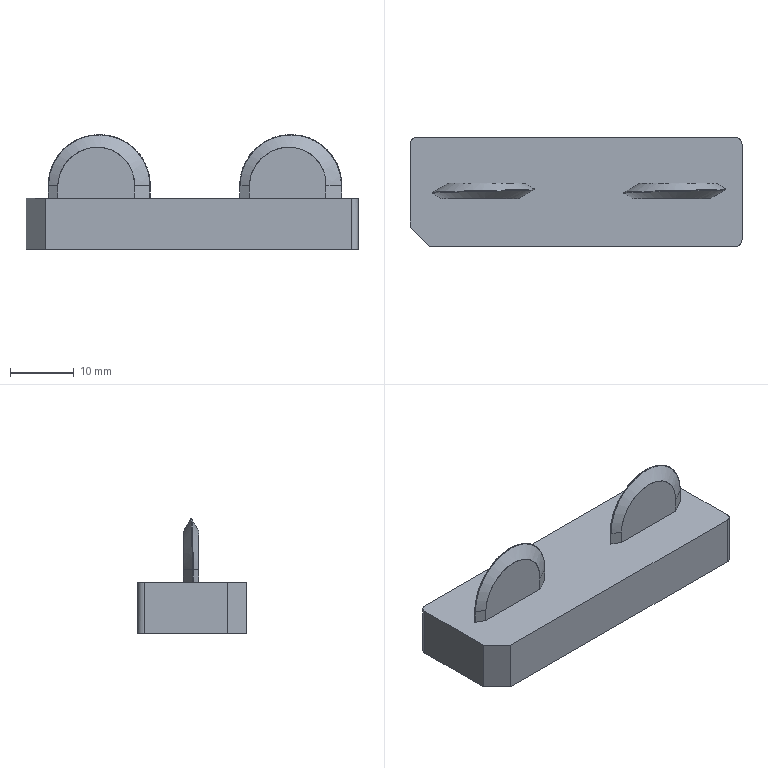NC program | PowerMill | posted with a generic post | part box 52 x 17 x 17.993 mm
Lines 4776 to 5766 of 175197:
N4873 M6
N4874 S18000 M03
N4875 G00 G90 X0.0 Y0.0
N4876 G43 Z9.812 H2
N4877
N4878 G05 P10000 R4
N4879 X-15.0046 Y3.2741
N4880 Z0.8142
N4881 G01 Z-0.3858 F3600.0
N4882 X-15.0151 Y3.2548 F6000.0
N4883 G03 X-14.9363 Y2.9861 I0.1738 J-0.0949
N4884 G01 X-13.6655 Y2.292
N4885 X-12.9334 Y2.2654
N4886 X-12.4453 Y2.2003
N4887 X-11.9573 Y2.0481
N4888 X-11.4692 Y1.7468
N4889 X-11.0258 Y1.2201
N4890 X-10.8183 Y0.7321
N4891 X-10.7493 Y0.244
N4892 X-10.7885 Y-0.244
N4893 X-10.9561 Y-0.7321
N4894 X-11.2918 Y-1.2201
N4895 X-11.4692 Y-1.3848
N4896 X-12.0007 Y-1.7082
N4897 X-12.4453 Y-1.8465
N4898 X-13.4214 Y-1.9746
N4899 X-14.3976 Y-2.0349
N4900 X-15.3737 Y-2.0324
N4901 X-16.3498 Y-1.9659
N4902 X-16.8378 Y-1.8637
N4903 X-17.3259 Y-1.6487
N4904 X-17.8296 Y-1.2201
N4905 X-18.1298 Y-0.7321
N4906 X-18.2691 Y-0.244
N4907 X-18.2928 Y0.244
N4908 X-18.2024 Y0.7321
N4909 X-17.974 Y1.2201
N4910 X-17.8139 Y1.4288
N4911 X-17.5262 Y1.7082
N4912 X-17.3259 Y1.8456
N4913 X-16.8378 Y2.0588
N4914 X-16.3498 Y2.1713
N4915 X-15.3737 Y2.2743
N4916 X-14.3976 Y2.3185
N4917 X-13.6655 Y2.292
N4918 X-15.0119 Y3.3954 Z-0.5837
N4919 X-15.0224 Y3.3761
N4920 G03 X-14.9438 Y3.1073 I0.1737 J-0.0951
N4921 G01 X-13.6613 Y2.4056
N4922 X-12.9334 Y2.3787
N4923 X-11.9573 Y2.2695
N4924 X-11.5961 Y2.1962
N4925 X-10.9812 Y1.929
N4926 X-10.6898 Y1.7082
N4927 X-10.4931 Y1.5014
N4928 X-10.2976 Y1.2201
N4929 X-10.1004 Y0.7321
N4930 X-10.0369 Y0.244
N4931 X-10.0778 Y-0.244
N4932 X-10.2499 Y-0.7321
N4933 X-10.5936 Y-1.2201
N4934 X-10.9812 Y-1.5344
N4935 X-11.3257 Y-1.7082
N4936 X-11.9573 Y-1.8834
N4937 X-13.4214 Y-2.087
N4938 X-14.3976 Y-2.149
N4939 X-15.3737 Y-2.1462
N4940 X-16.3498 Y-2.0801
N4941 X-17.3259 Y-1.9508
N4942 X-17.8139 Y-1.7872
N4943 X-17.9761 Y-1.7082
N4944 X-18.302 Y-1.4802
N4945 X-18.5591 Y-1.2201
N4946 X-18.79 Y-0.8714
N4947 X-18.8554 Y-0.7321
N4948 X-18.9931 Y-0.244
N4949 X-19.011 Y0.244
N4950 X-18.9164 Y0.7321
N4951 X-18.79 Y1.028
N4952 X-18.6799 Y1.2201
N4953 X-18.302 Y1.6425
N4954 X-17.8139 Y1.9476
N4955 X-17.3259 Y2.1163
N4956 X-16.3498 Y2.2825
N4957 X-15.3737 Y2.3875
N4958 X-14.3976 Y2.4329
N4959 X-13.6613 Y2.4056
N4960 X-14.9389 Y3.5136 Z-0.7815
N4961 X-14.9498 Y3.4945
N4962 G03 X-14.8755 Y3.2245 I0.1721 J-0.0978
N4963 G01 X-13.6546 Y2.5304
N4964 X-12.9334 Y2.492
N4965 X-11.9573 Y2.3804
N4966 X-10.9812 Y2.1908
N4967 X-10.4931 Y1.9775
N4968 X-10.1335 Y1.7082
N4969 X-10.0051 Y1.578
N4970 X-9.7514 Y1.2201
N4971 X-9.5544 Y0.7321
N4972 X-9.4932 Y0.244
N4973 X-9.5391 Y-0.244
N4974 X-9.7152 Y-0.7321
N4975 X-10.0051 Y-1.1528
N4976 X-10.4931 Y-1.5541
N4977 X-10.9812 Y-1.7729
N4978 X-11.9573 Y-1.992
N4979 X-13.3897 Y-2.1962
N4980 X-14.3976 Y-2.263
N4981 X-15.3737 Y-2.26
N4982 X-16.3095 Y-2.1962
N4983 X-17.8139 Y-1.9796
N4984 X-18.302 Y-1.8246
N4985 X-18.543 Y-1.7082
N4986 X-18.79 Y-1.5381
N4987 X-19.1129 Y-1.2201
N4988 X-19.2781 Y-0.9765
N4989 X-19.404 Y-0.7321
N4990 X-19.5376 Y-0.244
N4991 X-19.5511 Y0.244
N4992 X-19.4525 Y0.7321
N4993 X-19.213 Y1.2201
N4994 X-18.79 Y1.6717
N4995 X-18.302 Y1.9596
N4996 X-17.8139 Y2.1187
N4997 X-16.8378 Y2.3122
N4998 X-15.8617 Y2.4504
N4999 X-14.8856 Y2.5294
N5000 X-13.9095 Y2.544
N5001 X-13.6546 Y2.5304
N5002 X-15.0246 Y3.6221 Z-0.9794
N5003 X-15.0349 Y3.6026
N5004 G03 X-14.9531 Y3.3348 I0.1748 J-0.0929
N5005 G01 X-13.6518 Y2.6428
N5006 X-13.4214 Y2.637
N5007 X-12.4453 Y2.5528
N5008 X-11.4692 Y2.4064
N5009 X-10.4951 Y2.1962
N5010 X-10.0051 Y1.9658
N5011 X-9.6708 Y1.7082
N5012 X-9.517 Y1.5445
N5013 X-9.2943 Y1.2201
N5014 X-9.1039 Y0.7321
N5015 X-9.0457 Y0.244
N5016 X-9.094 Y-0.244
N5017 X-9.2715 Y-0.7321
N5018 X-9.517 Y-1.0997
N5019 X-9.6267 Y-1.2201
N5020 X-10.0051 Y-1.521
N5021 X-10.3719 Y-1.7082
N5022 X-10.9812 Y-1.8864
N5023 X-11.9573 Y-2.1006
N5024 X-12.5186 Y-2.1962
N5025 X-13.9095 Y-2.352
N5026 X-14.8856 Y-2.3811
N5027 X-15.8617 Y-2.345
N5028 X-16.8378 Y-2.2461
N5029 X-18.302 Y-1.9865
N5030 X-18.79 Y-1.8218
N5031 X-19.0097 Y-1.7082
N5032 X-19.2781 Y-1.5193
N5033 X-19.5727 Y-1.2201
N5034 X-19.7661 Y-0.9242
N5035 X-19.8572 Y-0.7321
N5036 X-19.9873 Y-0.244
N5037 X-19.9996 Y0.244
N5038 X-19.8987 Y0.7321
N5039 X-19.7661 Y1.0305
N5040 X-19.6537 Y1.2201
N5041 X-19.2781 Y1.6319
N5042 X-18.79 Y1.9358
N5043 X-18.302 Y2.1022
N5044 X-17.9373 Y2.1962
N5045 X-16.3498 Y2.5027
N5046 X-15.3737 Y2.6139
N5047 X-14.3976 Y2.6616
N5048 X-13.6518 Y2.6428
N5049 X-14.9229 Y3.7422 Z-1.1772
N5050 X-14.9339 Y3.7231
N5051 G03 X-14.8602 Y3.4529 I0.1719 J-0.0983
N5052 G01 X-13.6453 Y2.7583
N5053 X-12.9334 Y2.7186
N5054 X-11.9573 Y2.5999
N5055 X-10.9812 Y2.4215
N5056 X-10.0688 Y2.1962
N5057 X-9.517 Y1.9067
N5058 X-9.2762 Y1.7082
N5059 X-9.029 Y1.4178
N5060 X-8.9056 Y1.2201
N5061 X-8.7184 Y0.7321
N5062 X-8.6626 Y0.244
N5063 X-8.7131 Y-0.244
N5064 X-8.8936 Y-0.7321
N5065 X-9.029 Y-0.9521
N5066 X-9.2533 Y-1.2201
N5067 X-9.517 Y-1.4421
N5068 X-10.0014 Y-1.7082
N5069 X-10.4931 Y-1.8571
N5070 X-11.9011 Y-2.1962
N5071 X-12.4453 Y-2.293
N5072 X-13.4214 Y-2.4241
N5073 X-14.3976 Y-2.4911
N5074 X-15.3737 Y-2.4876
N5075 X-16.8378 Y-2.3583
N5076 X-17.8167 Y-2.1962
N5077 X-18.79 Y-1.9759
N5078 X-19.2781 Y-1.7835
N5079 X-19.4118 Y-1.7082
N5080 X-19.7661 Y-1.4373
N5081 X-19.9618 Y-1.2201
N5082 X-20.2437 Y-0.7321
N5083 X-20.3689 Y-0.244
N5084 X-20.3794 Y0.244
N5085 X-20.2776 Y0.7321
N5086 X-20.0298 Y1.2201
N5087 X-19.7661 Y1.5275
N5088 X-19.5506 Y1.7082
N5089 X-19.2781 Y1.8777
N5090 X-18.79 Y2.0704
N5091 X-17.8139 Y2.3278
N5092 X-16.8378 Y2.5312
N5093 X-15.8617 Y2.6752
N5094 X-14.8856 Y2.7584
N5095 X-13.9095 Y2.773
N5096 X-13.6453 Y2.7583
N5097 X-15.0115 Y3.8499 Z-1.375
N5098 X-15.0218 Y3.8305
N5099 G03 X-14.9403 Y3.5626 I0.1747 J-0.0932
N5100 G01 X-13.6424 Y2.8703
N5101 X-13.4214 Y2.8645
N5102 X-12.4453 Y2.7759
N5103 X-11.4692 Y2.6252
N5104 X-10.0051 Y2.2884
N5105 X-9.517 Y2.118
N5106 X-9.029 Y1.7992
N5107 X-8.9289 Y1.7082
N5108 X-8.563 Y1.2201
N5109 X-8.3772 Y0.7321
N5110 X-8.3236 Y0.244
N5111 X-8.3762 Y-0.244
N5112 X-8.5409 Y-0.6916
N5113 X-8.9247 Y-1.2201
N5114 X-9.029 Y-1.3164
N5115 X-9.517 Y-1.6372
N5116 X-10.0051 Y-1.8143
N5117 X-11.4168 Y-2.1962
N5118 X-12.4453 Y-2.4024
N5119 X-13.4214 Y-2.5365
N5120 X-14.3976 Y-2.6051
N5121 X-15.3737 Y-2.6014
N5122 X-16.3498 Y-2.5283
N5123 X-17.3259 Y-2.3913
N5124 X-18.2901 Y-2.1962
N5125 X-19.2781 Y-1.944
N5126 X-19.7665 Y-1.7082
N5127 X-20.2542 Y-1.2878
N5128 X-20.5848 Y-0.7321
N5129 X-20.7096 Y-0.244
N5130 X-20.7181 Y0.244
N5131 X-20.6136 Y0.7321
N5132 X-20.3609 Y1.2201
N5133 X-20.2542 Y1.3606
N5134 X-19.8777 Y1.7082
N5135 X-19.2781 Y2.0192
N5136 X-17.8139 Y2.433
N5137 X-16.8378 Y2.6408
N5138 X-15.3737 Y2.8403
N5139 X-14.3976 Y2.8902
N5140 X-13.6424 Y2.8703
N5141 X-14.9057 Y3.9702 Z-1.5729
N5142 X-14.9167 Y3.9511
N5143 G03 X-14.8437 Y3.6808 I0.1717 J-0.0987
N5144 G01 X-13.6356 Y2.9861
N5145 X-12.9334 Y2.9451
N5146 X-11.9573 Y2.8188
N5147 X-10.9812 Y2.6322
N5148 X-9.517 Y2.2486
N5149 X-9.029 Y2.0287
N5150 X-8.6121 Y1.7082
N5151 X-8.2504 Y1.2201
N5152 X-8.0686 Y0.7321
N5153 X-8.0168 Y0.244
N5154 X-8.0529 Y-0.1564
N5155 X-8.2568 Y-0.7321
N5156 X-8.5409 Y-1.1332
N5157 X-9.029 Y-1.53
N5158 X-9.3916 Y-1.7082
N5159 X-10.0051 Y-1.9112
N5160 X-11.4692 Y-2.3132
N5161 X-12.9334 Y-2.592
N5162 X-13.7845 Y-2.6843
N5163 X-14.3976 Y-2.7192
N5164 X-15.3737 Y-2.7152
N5165 X-16.3498 Y-2.6403
N5166 X-17.3259 Y-2.5007
N5167 X-18.7294 Y-2.1962
N5168 X-19.7661 Y-1.8838
N5169 X-20.2542 Y-1.5919
N5170 X-20.6201 Y-1.2201
N5171 X-20.7422 Y-1.0407
N5172 X-20.896 Y-0.7321
N5173 X-21.0187 Y-0.244
N5174 X-21.0241 Y0.244
N5175 X-20.9152 Y0.7321
N5176 X-20.6629 Y1.2201
N5177 X-20.2542 Y1.6469
N5178 X-19.7661 Y1.9418
N5179 X-19.2781 Y2.1132
N5180 X-17.8139 Y2.5375
N5181 X-16.8378 Y2.7503
N5182 X-15.8617 Y2.8999
N5183 X-14.8856 Y2.9873
N5184 X-13.9095 Y3.002
N5185 X-13.6356 Y2.9861
N5186 X-14.8953 Y4.0843 Z-1.7707
N5187 X-14.9063 Y4.0653
N5188 G03 X-14.8337 Y3.7948 I0.1716 J-0.099
N5189 G01 X-13.6289 Y3.0998
N5190 X-12.9334 Y3.0583
N5191 X-11.4692 Y2.8425
N5192 X-10.4931 Y2.6211
N5193 X-9.0647 Y2.1962
N5194 X-8.5409 Y1.8891
N5195 X-8.3324 Y1.7082
N5196 X-8.0529 Y1.3561
N5197 X-7.9745 Y1.2201
N5198 X-7.7948 Y0.7321
N5199 X-7.7451 Y0.244
N5200 X-7.8016 Y-0.244
N5201 X-7.9896 Y-0.7321
N5202 X-8.3611 Y-1.2201
N5203 X-8.5409 Y-1.3731
N5204 X-9.029 Y-1.6662
N5205 X-10.0051 Y-2.0062
N5206 X-11.4692 Y-2.419
N5207 X-12.8152 Y-2.6843
N5208 X-13.9095 Y-2.8067
N5209 X-14.8856 Y-2.8404
N5210 X-15.8617 Y-2.8013
N5211 X-16.8378 Y-2.6915
N5212 X-18.302 Y-2.4037
N5213 X-19.7661 Y-1.9919
N5214 X-20.2542 Y-1.7841
N5215 X-20.7422 Y-1.4083
N5216 X-20.904 Y-1.2201
N5217 X-21.175 Y-0.7321
N5218 X-21.2957 Y-0.244
N5219 X-21.2995 Y0.244
N5220 X-21.1875 Y0.7321
N5221 X-20.9332 Y1.2201
N5222 X-20.7422 Y1.4473
N5223 X-20.4369 Y1.7082
N5224 X-20.2542 Y1.8265
N5225 X-19.7661 Y2.039
N5226 X-18.79 Y2.365
N5227 X-17.6373 Y2.6843
N5228 X-16.8378 Y2.8593
N5229 X-15.8617 Y3.0122
N5230 X-14.8856 Y3.1018
N5231 X-13.9095 Y3.1165
N5232 X-13.6289 Y3.0998
N5233 X-14.989 Y4.1916 Z-1.9686
N5234 X-14.9994 Y4.1722
N5235 G03 X-14.9184 Y3.9041 I0.1745 J-0.0936
N5236 G01 X-13.6257 Y3.2114
N5237 X-13.4214 Y3.2056
N5238 X-12.4453 Y3.1127
N5239 X-11.4692 Y2.9486
N5240 X-10.0051 Y2.5892
N5241 X-8.7876 Y2.1962
N5242 X-8.5409 Y2.0726
N5243 X-8.0693 Y1.7082
N5244 X-7.7155 Y1.2201
N5245 X-7.5648 Y0.8348
N5246 X-7.49 Y0.244
N5247 X-7.5485 Y-0.244
N5248 X-7.7401 Y-0.7321
N5249 X-8.0529 Y-1.1592
N5250 X-8.5409 Y-1.5439
N5251 X-8.8943 Y-1.7082
N5252 X-9.517 Y-1.934
N5253 X-10.9812 Y-2.3943
N5254 X-12.19 Y-2.6843
N5255 X-13.4214 Y-2.8738
N5256 X-14.3976 Y-2.9479
N5257 X-15.3737 Y-2.9427
N5258 X-16.3498 Y-2.8644
N5259 X-17.5208 Y-2.6843
N5260 X-18.79 Y-2.3805
N5261 X-20.2542 Y-1.9215
N5262 X-20.6467 Y-1.7082
N5263 X-21.1618 Y-1.2201
N5264 X-21.4297 Y-0.7321
N5265 X-21.5482 Y-0.244
N5266 X-21.5506 Y0.244
N5267 X-21.4397 Y0.7321
N5268 X-21.2303 Y1.1463
N5269 X-20.7422 Y1.6627
N5270 X-20.2542 Y1.9485
N5271 X-19.7661 Y2.1283
N5272 X-18.302 Y2.6044
N5273 X-16.8378 Y2.9664
N5274 X-15.4409 Y3.1723
N5275 X-14.3976 Y3.2332
N5276 X-13.6257 Y3.2114
N5277 X-14.9848 Y4.3035 Z-2.1664
N5278 X-14.9952 Y4.2841
N5279 G03 X-14.9138 Y4.0162 I0.1747 J-0.0932
N5280 G01 X-13.6226 Y3.3268
N5281 X-13.4214 Y3.3214
N5282 X-12.4453 Y3.2251
N5283 X-10.9812 Y2.9482
N5284 X-9.9939 Y2.6843
N5285 X-8.5343 Y2.1962
N5286 X-8.0529 Y1.9086
N5287 X-7.8259 Y1.7082
N5288 X-7.5648 Y1.3766
N5289 X-7.4761 Y1.2201
N5290 X-7.3004 Y0.7321
N5291 X-7.2538 Y0.244
N5292 X-7.3146 Y-0.244
N5293 X-7.5065 Y-0.7321
N5294 X-7.885 Y-1.2201
N5295 X-8.0529 Y-1.3636
N5296 X-8.5409 Y-1.6546
N5297 X-9.029 Y-1.8459
N5298 X-10.4931 Y-2.3502
N5299 X-11.7131 Y-2.6843
N5300 X-12.9334 Y-2.9243
N5301 X-13.9095 Y-3.034
N5302 X-14.8856 Y-3.0707
N5303 X-15.8617 Y-3.0278
N5304 X-16.8378 Y-2.9106
N5305 X-17.8139 Y-2.7237
N5306 X-18.79 Y-2.4804
N5307 X-20.2542 Y-2.0157
N5308 X-20.7422 Y-1.8028
N5309 X-20.8912 Y-1.7082
N5310 X-21.2303 Y-1.4225
N5311 X-21.4016 Y-1.2201
N5312 X-21.6668 Y-0.7321
N5313 X-21.7834 Y-0.244
N5314 X-21.7847 Y0.244
N5315 X-21.6702 Y0.7321
N5316 X-21.4088 Y1.2201
N5317 X-21.2303 Y1.4321
N5318 X-20.9088 Y1.7082
N5319 X-20.7422 Y1.8152
N5320 X-20.2542 Y2.0349
N5321 X-18.79 Y2.5556
N5322 X-17.3259 Y2.9645
N5323 X-16.3498 Y3.1613
N5324 X-15.3737 Y3.2925
N5325 X-14.3976 Y3.3476
N5326 X-13.6226 Y3.3268
N5327 X-15.0437 Y4.3373 Z-2.3642
N5328 X-15.0535 Y4.3176
N5329 G03 X-14.965 Y4.0519 I0.1771 J-0.0886
N5330 G01 X-13.6226 Y3.3808
N5331 X-12.9334
N5332 X-12.4453 Y3.3341
N5333 X-11.9573 Y3.2566
N5334 X-10.9812 Y3.0522
N5335 X-9.6826 Y2.6843
N5336 X-8.2972 Y2.1962
N5337 X-8.0529 Y2.0685
N5338 X-7.6051 Y1.7082
N5339 X-7.2579 Y1.2201
N5340 X-7.0848 Y0.7321
N5341 X-7.0398 Y0.244
N5342 X-7.1019 Y-0.244
N5343 X-7.2959 Y-0.7321
N5344 X-7.5648 Y-1.1042
N5345 X-7.6778 Y-1.2201
N5346 X-8.0529 Y-1.5111
N5347 X-8.4659 Y-1.7082
N5348 X-10.0051 Y-2.2879
N5349 X-11.3048 Y-2.6843
N5350 X-11.9573 Y-2.8455
N5351 X-12.9334 Y-3.0348
N5352 X-13.4214 Y-3.0748
N5353 X-16.3498 Y-3.0731
N5354 X-16.8378 Y-3.0228
N5355 X-17.3259 Y-2.9379
N5356 X-18.302 Y-2.7167
N5357 X-19.2781 Y-2.4335
N5358 X-20.7422 Y-1.9218
N5359 X-21.2303 Y-1.6261
N5360 X-21.6259 Y-1.2201
N5361 X-21.7183 Y-1.0821
N5362 X-21.8884 Y-0.7321
N5363 X-22.0033 Y-0.244
N5364 X-22.002 Y0.244
N5365 X-21.8874 Y0.7321
N5366 X-21.7183 Y1.0769
N5367 X-21.6237 Y1.2201
N5368 X-21.2303 Y1.6238
N5369 X-21.1208 Y1.7082
N5370 X-20.7422 Y1.9215
N5371 X-19.2781 Y2.4839
N5372 X-18.302 Y2.8049
N5373 X-16.8378 Y3.1806
N5374 X-15.8617 Y3.3493
N5375 X-15.3737 Y3.3808
N5376 X-13.6226
N5377 X-15.0582 Y4.3445 Z-2.5621
N5378 X-15.068 Y4.3248
N5379 G03 X-14.9795 Y4.0591 I0.1771 J-0.0886
N5380 G01 X-13.6226 Y3.3807
N5381 X-12.9334
N5382 X-12.9231 Y3.3797
N5383 X-12.9135
N5384 X-12.4352 Y3.3807
N5385 X-11.9573 Y3.361
N5386 X-11.0481 Y3.1723
N5387 X-9.517 Y2.7259
N5388 X-8.0529 Y2.1844
N5389 X-7.5648 Y1.8682
N5390 X-7.3919 Y1.7082
N5391 X-7.0768 Y1.275
N5392 X-6.8767 Y0.7321
N5393 X-6.8332 Y0.244
N5394 X-6.8974 Y-0.244
N5395 X-7.0768 Y-0.7004
N5396 X-7.4786 Y-1.2201
N5397 X-8.0529 Y-1.6139
N5398 X-9.517 Y-2.2019
N5399 X-10.9509 Y-2.6843
N5400 X-11.4692 Y-2.8304
N5401 X-12.4453 Y-3.0529
N5402 X-12.9334 Y-3.0748
N5403 X-16.8378
N5404 X-17.3259 Y-3.0402
N5405 X-18.302 Y-2.817
N5406 X-19.2781 Y-2.5279
N5407 X-20.7422 Y-2.0094
N5408 X-21.2303 Y-1.7807
N5409 X-21.7183 Y-1.3648
N5410 X-21.8343 Y-1.2201
N5411 X-22.0943 Y-0.7321
N5412 X-22.2064 Y-0.2542
N5413 Y0.2413
N5414 X-22.0884 Y0.7321
N5415 X-21.8227 Y1.2201
N5416 X-21.7183 Y1.3494
N5417 X-21.3161 Y1.7082
N5418 X-20.7422 Y1.9988
N5419 X-19.7661 Y2.3918
N5420 X-18.302 Y2.9017
N5421 X-17.3352 Y3.1723
N5422 X-16.3498 Y3.3716
N5423 X-15.4827 Y3.3737
N5424 X-15.3737 Y3.3807
N5425 X-13.6226
N5426 X-15.0607 Y4.3458 Z-2.7599
N5427 X-15.0705 Y4.3261
N5428 G03 X-14.982 Y4.0605 I0.1771 J-0.0885
N5429 G01 X-13.6226 Y3.3808
N5430 X-11.9573
N5431 X-11.4692 Y3.3633
N5432 X-10.4931 Y3.1264
N5433 X-9.517 Y2.8172
N5434 X-7.874 Y2.1962
N5435 X-7.5648 Y2.0201
N5436 X-7.1992 Y1.7082
N5437 X-7.0768 Y1.5657
N5438 X-6.8582 Y1.2201
N5439 X-6.6891 Y0.7321
N5440 X-6.6471 Y0.244
N5441 X-6.7125 Y-0.244
N5442 X-6.9103 Y-0.7321
N5443 X-7.0768 Y-0.9795
N5444 X-7.2989 Y-1.2201
N5445 X-7.5648 Y-1.4363
N5446 X-8.0529 Y-1.6896
N5447 X-9.029 Y-2.0968
N5448 X-10.6362 Y-2.6843
N5449 X-10.9812 Y-2.7917
N5450 X-11.9573 Y-3.0481
N5451 X-12.4453 Y-3.0748
N5452 X-17.3259
N5453 X-17.8139 Y-3.0403
N5454 X-18.302 Y-2.9169
N5455 X-19.7661 Y-2.4594
N5456 X-21.2303 Y-1.8919
N5457 X-21.5345 Y-1.7082
N5458 X-21.7183 Y-1.5582
N5459 X-22.0262 Y-1.2201
N5460 X-22.2064 Y-0.9149
N5461 X-22.2844 Y-0.7321
N5462 X-22.3951 Y-0.244
N5463 X-22.3926 Y0.244
N5464 X-22.2736 Y0.7321
N5465 X-22.2064 Y0.8859
N5466 X-22.005 Y1.2201
N5467 X-21.7183 Y1.5293
N5468 X-21.4965 Y1.7082
N5469 X-21.2303 Y1.864
N5470 X-19.7661 Y2.4781
N5471 X-18.79 Y2.8358
N5472 X-17.3259 Y3.2766
N5473 X-16.8378 Y3.3721
N5474 X-16.3498 Y3.3808
N5475 X-13.6226
N5476 X-15.0606 Y4.3458 Z-2.9578
N5477 X-15.0704 Y4.3261
N5478 G03 X-14.9819 Y4.0604 I0.1771 J-0.0886
N5479 G01 X-13.6226 Y3.3808
N5480 X-12.7821
N5481 X-11.9573
N5482 X-11.9569
N5483 X-11.4692 Y3.3807
N5484 X-10.9812 Y3.3502
N5485 X-10.0051 Y3.0723
N5486 X-8.5409 Y2.5474
N5487 X-7.5648 Y2.1358
N5488 X-7.0768 Y1.769
N5489 X-6.6781 Y1.2201
N5490 X-6.5887 Y1.0103
N5491 X-6.5108 Y0.7321
N5492 X-6.4701 Y0.244
N5493 X-6.5363 Y-0.244
N5494 X-6.7368 Y-0.7321
N5495 X-7.0768 Y-1.172
N5496 X-7.5648 Y-1.5402
N5497 X-9.029 Y-2.1805
N5498 X-10.3611 Y-2.6843
N5499 X-11.4692 Y-3.0278
N5500 X-11.9573 Y-3.0748
N5501 X-17.8139
N5502 X-18.302 Y-3.0179
N5503 X-19.3795 Y-2.6843
N5504 X-21.2303 Y-1.9779
N5505 X-21.7245 Y-1.7082
N5506 X-22.2085 Y-1.2201
N5507 X-22.4632 Y-0.7321
N5508 X-22.5731 Y-0.244
N5509 X-22.5694 Y0.244
N5510 X-22.4478 Y0.7321
N5511 X-22.2064 Y1.182
N5512 X-21.7183 Y1.6715
N5513 X-21.2303 Y1.9408
N5514 X-19.449 Y2.6843
N5515 X-18.0558 Y3.1723
N5516 X-17.3259 Y3.3617
N5517 X-16.8378 Y3.3808
N5518 X-13.6226
N5519 X-15.0574 Y4.3441 Z-3.1556
N5520 X-15.0673 Y4.3245
N5521 G03 X-14.9787 Y4.0588 I0.1771 J-0.0886
N5522 G01 X-13.6226 Y3.3808
N5523 X-10.9812
N5524 X-10.4931 Y3.3195
N5525 X-9.029 Y2.8208
N5526 X-7.5008 Y2.1962
N5527 X-7.0768 Y1.9256
N5528 X-6.8433 Y1.7082
N5529 X-6.5887 Y1.3691
N5530 X-6.5084 Y1.2201
N5531 X-6.343 Y0.7321
N5532 X-6.3038 Y0.244
N5533 X-6.3707 Y-0.244
N5534 X-6.574 Y-0.7321
N5535 X-6.9671 Y-1.2201
N5536 X-7.0768 Y-1.3161
N5537 X-7.5648 Y-1.6164
N5538 X-9.029 Y-2.261
N5539 X-10.1109 Y-2.6843
N5540 X-10.9812 Y-2.9838
N5541 X-11.4692 Y-3.0704
N5542 X-11.9573 Y-3.0748
N5543 X-17.8139
N5544 X-18.302 Y-3.0687
N5545 X-18.79 Y-2.9719
N5546 X-19.2781 Y-2.8112
N5547 X-20.7422 Y-2.2569
N5548 X-21.7183 Y-1.8296
N5549 X-21.9002 Y-1.7082
N5550 X-22.2064 Y-1.4333
N5551 X-22.3798 Y-1.2201
N5552 X-22.6339 Y-0.7321
N5553 X-22.6945 Y-0.5287
N5554 X-22.742 Y-0.244
N5555 X-22.7359 Y0.244
N5556 X-22.614 Y0.7321
N5557 X-22.3414 Y1.2201
N5558 X-22.2064 Y1.3794
N5559 X-21.8266 Y1.7082
N5560 X-21.7183 Y1.7766
N5561 X-20.2542 Y2.4399
N5562 X-18.79 Y3.0175
N5563 X-17.8139 Y3.3341
N5564 X-17.3259 Y3.3807
N5565 X-16.839 Y3.3808
N5566 X-16.8378
N5567 X-15.0874
N5568 X-13.6226
N5569 X-15.0613 Y4.3461 Z-3.3534
N5570 X-15.0711 Y4.3264
N5571 G03 X-14.9826 Y4.0608 I0.1771 J-0.0885
N5572 G01 X-13.6226 Y3.3808
N5573 X-10.9812
N5574 X-10.4931 Y3.3695
N5575 X-10.0051 Y3.261
N5576 X-9.029 Y2.9051
N5577 X-7.3325 Y2.1962
N5578 X-7.0768 Y2.0478
N5579 X-6.6851 Y1.7082
N5580 X-6.5887 Y1.5941
N5581 X-6.3528 Y1.2201
N5582 X-6.1881 Y0.7321
N5583 X-6.15 Y0.244
N5584 X-6.2198 Y-0.244
N5585 X-6.4233 Y-0.7321
N5586 X-6.5887 Y-0.9743
N5587 X-6.818 Y-1.2201
N5588 X-7.0768 Y-1.4274
N5589 X-8.0529 Y-1.9098
N5590 X-9.8802 Y-2.6843
N5591 X-10.4931 Y-2.9117
N5592 X-10.9812 Y-3.0484
N5593 X-11.4692 Y-3.0748
N5594 X-18.302
N5595 X-18.79 Y-3.0433
N5596 X-19.2781 Y-2.9032
N5597 X-20.2542 Y-2.5377
N5598 X-21.7183 Y-1.9175
N5599 X-22.0626 Y-1.7082
N5600 X-22.2064 Y-1.5882
N5601 X-22.538 Y-1.2201
N5602 X-22.6945 Y-0.9562
N5603 X-22.7888 Y-0.7321
N5604 X-22.8958 Y-0.244
N5605 X-22.8888 Y0.244
N5606 X-22.7646 Y0.7321
N5607 X-22.6945 Y0.891
N5608 X-22.4899 Y1.2201
N5609 X-22.2064 Y1.5248
N5610 X-21.9742 Y1.7082
N5611 X-21.7183 Y1.8551
N5612 X-20.9842 Y2.1962
N5613 X-19.2781 Y2.922
N5614 X-18.302 Y3.2785
N5615 X-17.8139 Y3.3755
N5616 X-17.3259 Y3.3808
N5617 X-13.6226
N5618 X-15.0613 Y4.3461 Z-3.5513
N5619 X-15.0712 Y4.3264
N5620 G03 X-14.9826 Y4.0608 I0.1771 J-0.0885
N5621 G01 X-13.6226 Y3.3808
N5622 X-10.4931
N5623 X-10.0051 Y3.335
N5624 X-9.517 Y3.1783
N5625 X-8.5409 Y2.7934
N5626 X-7.0768 Y2.1443
N5627 X-6.5887 Y1.7656
N5628 X-6.2024 Y1.2201
N5629 X-6.1007 Y0.9628
N5630 X-6.0403 Y0.7321
N5631 X-6.0034 Y0.244
N5632 X-6.0742 Y-0.244
N5633 X-6.2796 Y-0.7321
N5634 X-6.5887 Y-1.1335
N5635 X-7.0768 Y-1.513
N5636 X-8.5409 Y-2.2021
N5637 X-9.6707 Y-2.6843
N5638 X-10.4931 Y-2.9968
N5639 X-10.9812 Y-3.0721
N5640 X-11.4208
N5641 X-11.4692 Y-3.0748
N5642 X-18.302
N5643 X-18.3388 Y-3.0724
N5644 X-18.3451
N5645 X-18.79
N5646 X-19.2781 Y-2.9899
N5647 X-19.7661 Y-2.8107
N5648 X-21.7183 Y-1.9918
N5649 X-22.2179 Y-1.7082
N5650 X-22.6883 Y-1.2201
N5651 X-22.9385 Y-0.7321
N5652 X-23.0435 Y-0.244
N5653 X-23.0344 Y0.244
N5654 X-22.9101 Y0.7321
N5655 X-22.6334 Y1.2201
N5656 X-22.2064 Y1.6399
N5657 X-21.7183 Y1.9204
N5658 X-20.0468 Y2.6843
N5659 X-18.79 Y3.1936
N5660 X-18.302 Y3.3445
N5661 X-17.8139 Y3.3808
N5662 X-13.6226
N5663 X-15.0548 Y4.3428 Z-3.7491
N5664 X-15.0646 Y4.3231
N5665 G03 X-14.976 Y4.0575 I0.1771 J-0.0885
N5666 G01 X-13.6226 Y3.3808
N5667 X-10.4931
N5668 X-10.0051 Y3.3714
N5669 X-9.517 Y3.2634
N5670 X-8.5409 Y2.8713
N5671 X-7.0253 Y2.1962
N5672 X-6.5887 Y1.9009
N5673 X-6.3927 Y1.7082
N5674 X-6.1007 Y1.2933
N5675 X-5.9038 Y0.7321
N5676 X-5.8685 Y0.244
N5677 X-5.9397 Y-0.244
N5678 X-6.1007 Y-0.6488
N5679 X-6.5473 Y-1.2201
N5680 X-7.0768 Y-1.5771
N5681 X-7.5648 Y-1.8142
N5682 X-9.4778 Y-2.6843
N5683 X-10.0051 Y-2.9025
N5684 X-10.4931 Y-3.0465
N5685 X-10.9812 Y-3.0748
N5686 X-18.79
N5687 X-19.2781 Y-3.0439
N5688 X-19.7661 Y-2.8978
N5689 X-21.2303 Y-2.283
N5690 X-22.2064 Y-1.818
N5691 X-22.3631 Y-1.7082
N5692 X-22.6945 Y-1.3927
N5693 X-22.8293 Y-1.2201
N5694 X-23.0761 Y-0.7321
N5695 X-23.1804 Y-0.244
N5696 X-23.1825 Y0.1286
N5697 X-23.0442 Y0.7321
N5698 X-22.7654 Y1.2201
N5699 X-22.2428 Y1.7082
N5700 X-21.7183 Y1.9825
N5701 X-20.2143 Y2.6843
N5702 X-18.79 Y3.2766
N5703 X-18.302 Y3.3746
N5704 X-17.8139 Y3.3808
N5705 X-13.6226
N5706 X-15.0613 Y4.3461 Z-3.947
N5707 X-15.0712 Y4.3264
N5708 G03 X-14.9826 Y4.0608 I0.1771 J-0.0885
N5709 G01 X-13.6226 Y3.3808
N5710 X-10.0051 Y3.3807
N5711 X-9.517 Y3.3273
N5712 X-9.0707 Y3.1723
N5713 X-8.5409 Y2.9493
N5714 X-6.887 Y2.1962
N5715 X-6.5887 Y2.0102
N5716 X-6.2595 Y1.7082
N5717 X-6.1007 Y1.5075
N5718 X-5.9337 Y1.2201
N5719 X-5.7751 Y0.7321
N5720 X-5.7408 Y0.244
N5721 X-5.814 Y-0.244
N5722 X-6.0228 Y-0.7321
N5723 X-6.1007 Y-0.853
N5724 X-6.4252 Y-1.2201
N5725 X-6.5887 Y-1.3561
N5726 X-7.0768 Y-1.6378
N5727 X-9.3013 Y-2.6843
N5728 X-10.0051 Y-2.9749
N5729 X-10.4931 Y-3.0695
N5730 X-10.9812 Y-3.0748
N5731 X-18.79
N5732 X-19.2781 Y-3.0696
N5733 X-19.7661 Y-2.9752
N5734 X-20.2542 Y-2.7778
N5735 X-22.2064 Y-1.8971
N5736 X-22.4987 Y-1.7082
N5737 X-22.6945 Y-1.5341
N5738 X-22.9597 Y-1.2201
N5739 X-23.1825 Y-0.7937
N5740 X-23.3071 Y-0.244
N5741 X-23.2964 Y0.244
N5742 X-23.1825 Y0.6951
N5743 X-22.8866 Y1.2201
N5744 X-22.6945 Y1.4342
N5745 X-22.361 Y1.7082
N5746 X-22.2064 Y1.7997
N5747 X-20.375 Y2.6843
N5748 X-19.2627 Y3.1723
N5749 X-18.79 Y3.3338
N5750 X-18.302 Y3.3808
N5751 X-13.6226
N5752 X-15.0613 Y4.3461 Z-4.1448
N5753 X-15.0712 Y4.3264
N5754 G03 X-14.9826 Y4.0608 I0.1771 J-0.0885
N5755 G01 X-13.6226 Y3.3808
N5756 X-10.0051 Y3.3807
N5757 X-9.517 Y3.3626
N5758 X-9.029 Y3.2325
N5759 X-7.782 Y2.6843
N5760 X-6.5887 Y2.1008
N5761 X-6.1332 Y1.7082
N5762 X-5.8091 Y1.2201
N5763 X-5.6524 Y0.7321
N5764 X-5.6197 Y0.244
N5765 X-5.6935 Y-0.244
N5766 X-5.904 Y-0.7321
N5767 X-6.1007 Y-1.0045
N5768 X-6.3088 Y-1.2201
N5769 X-6.5887 Y-1.4357
N5770 X-7.1079 Y-1.7082
N5771 X-9.1378 Y-2.6843
N5772 X-9.517 Y-2.8546
N5773 X-10.0051 Y-3.0248
N5774 X-10.4931 Y-3.0748
N5775 X-19.2781
N5776 X-19.7661 Y-3.0274
N5777 X-20.2542 Y-2.8578
N5778 X-22.2064 Y-1.9633
N5779 X-22.6285 Y-1.7082
N5780 X-23.0833 Y-1.2201
N5781 X-23.1825 Y-1.0579
N5782 X-23.3264 Y-0.7321
N5783 X-23.4275 Y-0.244
N5784 X-23.4154 Y0.244
N5785 X-23.2861 Y0.7321
N5786 X-23.1825 Y0.9481
N5787 X-23.0029 Y1.2201
N5788 X-22.6945 Y1.5411
N5789 X-22.473 Y1.7082
N5790 X-20.7422 Y2.5793
N5791 X-19.2781 Y3.2406
N5792 X-18.79 Y3.3643
N5793 X-18.302 Y3.3808
N5794 X-13.6226
N5795 X-15.0615 Y4.3461 Z-4.3426
N5796 X-15.0713 Y4.3265
N5797 G03 X-14.9827 Y4.0608 I0.1771 J-0.0886
N5798 G01 X-13.6226 Y3.3807
N5799 X-10.0051
N5800 X-9.9496 Y3.3786
N5801 X-9.946
N5802 X-9.517
N5803 X-9.029 Y3.2968
N5804 X-8.7058 Y3.1723
N5805 X-6.6318 Y2.1962
N5806 X-6.1007 Y1.7959
N5807 X-6.0176 Y1.7082
N5808 X-5.6967 Y1.2201
N5809 X-5.6126 Y1.0071
N5810 X-5.5408 Y0.7321
N5811 X-5.5087 Y0.244
N5812 X-5.585 Y-0.244
N5813 X-5.798 Y-0.7321
N5814 X-6.2031 Y-1.2201
N5815 X-6.5887 Y-1.4964
N5816 X-8.9885 Y-2.6843
N5817 X-9.517 Y-2.9242
N5818 X-10.0051 Y-3.0553
N5819 X-10.4931 Y-3.0748
N5820 X-19.2781
N5821 X-19.7661 Y-3.0578
N5822 X-20.2542 Y-2.9332
N5823 X-22.2064 Y-2.0261
N5824 X-22.6945 Y-1.7491
N5825 X-23.1825 Y-1.2464
N5826 X-23.4428 Y-0.7321
N5827 X-23.5421 Y-0.244
N5828 X-23.5292 Y0.244
N5829 X-23.3981 Y0.7321
N5830 X-23.1134 Y1.2201
N5831 X-22.6945 Y1.6292
N5832 X-22.581 Y1.7082
N5833 X-21.2303 Y2.4036
N5834 X-19.6114 Y3.1723
N5835 X-19.2781 Y3.3004
N5836 X-18.79 Y3.3789
N5837 X-18.3582
N5838 X-18.302 Y3.3808
N5839 X-13.6226 Y3.3807
N5840 X-15.0596 Y4.3453 Z-4.5405
N5841 X-15.0694 Y4.3256
N5842 G03 X-14.9809 Y4.06 I0.1771 J-0.0886
N5843 G01 X-13.6226 Y3.3808
N5844 X-9.517
N5845 X-9.029 Y3.338
N5846 X-8.543 Y3.1723
N5847 X-6.5155 Y2.1962
N5848 X-6.1007 Y1.9059
N5849 X-5.9063 Y1.7082
N5850 X-5.6126 Y1.2716
N5851 X-5.4333 Y0.7321
N5852 X-5.4023 Y0.244
N5853 X-5.4799 Y-0.244
N5854 X-5.6126 Y-0.5846
N5855 X-5.6937 Y-0.7321
N5856 X-6.1014 Y-1.2201
N5857 X-6.5887 Y-1.5477
N5858 X-8.843 Y-2.6843
N5859 X-9.517 Y-2.9785
N5860 X-10.0051 Y-3.0703
N5861 X-10.2492 Y-3.0677
N5862 X-10.4931 Y-3.0748
N5863 X-19.2781